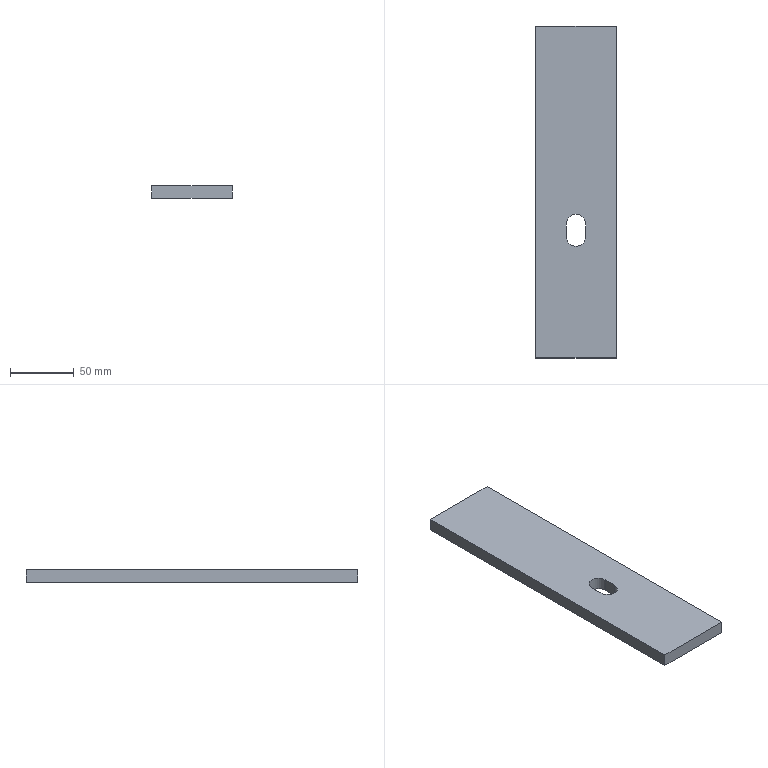Part | STEP file | E3-计量楼梯连接Plate 1 | 1 solid | 10 faces | box 63 x 260 x 10 mm | volume 160533 mm3 | plane 8 | cylinder 2 | commonest cylinder face diameters 15 x2
STEP:
#1=CARTESIAN_POINT('',(0.,0.,0.));
#2=DIRECTION('',(0.,0.,1.));
#3=DIRECTION('',(1.,0.,0.));
#4=AXIS2_PLACEMENT_3D('',#1,#2,#3);
#5=CARTESIAN_POINT('',(-31.5,260.,0.));
#6=VERTEX_POINT('',#5);
#7=CARTESIAN_POINT('',(-31.5,0.,0.));
#8=VERTEX_POINT('',#7);
#9=CARTESIAN_POINT('',(-31.5,260.,0.));
#10=DIRECTION('',(0.,-1.,0.));
#11=VECTOR('',#10,1.);
#12=LINE('',#9,#11);
#13=CARTESIAN_POINT('',(-31.5,260.,-10.));
#14=DIRECTION('',(1.,0.,0.));
#15=DIRECTION('',(0.,1.,0.));
#16=AXIS2_PLACEMENT_3D('',#13,#14,#15);
#17=PLANE('',#16);
#18=CARTESIAN_POINT('',(0.,10.));
#19=DIRECTION('',(-1.,0.));
#20=VECTOR('',#19,1.);
#21=LINE('',#18,#20);
#22=(GEOMETRIC_REPRESENTATION_CONTEXT(2)PARAMETRIC_REPRESENTATION_CONTEXT()REPRESENTATION_CONTEXT('',''));
#23=DEFINITIONAL_REPRESENTATION('',(#21),#22);
#24=PCURVE('',#17,#23);
#25=CARTESIAN_POINT('',(0.,0.,0.));
#26=DIRECTION('',(0.,0.,-1.));
#27=DIRECTION('',(1.,0.,0.));
#28=AXIS2_PLACEMENT_3D('',#25,#26,#27);
#29=PLANE('',#28);
#30=CARTESIAN_POINT('',(-31.5,-260.));
#31=DIRECTION('',(0.,1.));
#32=VECTOR('',#31,1.);
#33=LINE('',#30,#32);
#34=(GEOMETRIC_REPRESENTATION_CONTEXT(2)PARAMETRIC_REPRESENTATION_CONTEXT()REPRESENTATION_CONTEXT('',''));
#35=DEFINITIONAL_REPRESENTATION('',(#33),#34);
#36=PCURVE('',#29,#35);
#37=SURFACE_CURVE('',#12,(#24,#36),.PCURVE_S1.);
#38=EDGE_CURVE('',#6,#8,#37,.T.);
#39=ORIENTED_EDGE('',*,*,#38,.F.);
#40=CARTESIAN_POINT('',(-31.5,260.,-10.));
#41=VERTEX_POINT('',#40);
#42=CARTESIAN_POINT('',(-31.5,260.,-10.));
#43=DIRECTION('',(0.,0.,1.));
#44=VECTOR('',#43,1.);
#45=LINE('',#42,#44);
#46=CARTESIAN_POINT('',(0.,0.));
#47=DIRECTION('',(0.,1.));
#48=VECTOR('',#47,1.);
#49=LINE('',#46,#48);
#50=(GEOMETRIC_REPRESENTATION_CONTEXT(2)PARAMETRIC_REPRESENTATION_CONTEXT()REPRESENTATION_CONTEXT('',''));
#51=DEFINITIONAL_REPRESENTATION('',(#49),#50);
#52=PCURVE('',#17,#51);
#53=CARTESIAN_POINT('',(-31.5,260.,-10.));
#54=DIRECTION('',(0.,-1.,0.));
#55=DIRECTION('',(0.,0.,1.));
#56=AXIS2_PLACEMENT_3D('',#53,#54,#55);
#57=PLANE('',#56);
#58=CARTESIAN_POINT('',(0.,0.));
#59=DIRECTION('',(1.,0.));
#60=VECTOR('',#59,1.);
#61=LINE('',#58,#60);
#62=(GEOMETRIC_REPRESENTATION_CONTEXT(2)PARAMETRIC_REPRESENTATION_CONTEXT()REPRESENTATION_CONTEXT('',''));
#63=DEFINITIONAL_REPRESENTATION('',(#61),#62);
#64=PCURVE('',#57,#63);
#65=SURFACE_CURVE('',#45,(#52,#64),.PCURVE_S1.);
#66=EDGE_CURVE('',#41,#6,#65,.T.);
#67=ORIENTED_EDGE('',*,*,#66,.F.);
#68=CARTESIAN_POINT('',(-31.5,0.,-10.));
#69=VERTEX_POINT('',#68);
#70=CARTESIAN_POINT('',(-31.5,260.,-10.));
#71=DIRECTION('',(0.,-1.,0.));
#72=VECTOR('',#71,1.);
#73=LINE('',#70,#72);
#74=CARTESIAN_POINT('',(0.,0.));
#75=DIRECTION('',(-1.,0.));
#76=VECTOR('',#75,1.);
#77=LINE('',#74,#76);
#78=(GEOMETRIC_REPRESENTATION_CONTEXT(2)PARAMETRIC_REPRESENTATION_CONTEXT()REPRESENTATION_CONTEXT('',''));
#79=DEFINITIONAL_REPRESENTATION('',(#77),#78);
#80=PCURVE('',#17,#79);
#81=CARTESIAN_POINT('',(0.,0.,-10.));
#82=DIRECTION('',(0.,0.,-1.));
#83=DIRECTION('',(1.,0.,0.));
#84=AXIS2_PLACEMENT_3D('',#81,#82,#83);
#85=PLANE('',#84);
#86=CARTESIAN_POINT('',(-31.5,-260.));
#87=DIRECTION('',(0.,1.));
#88=VECTOR('',#87,1.);
#89=LINE('',#86,#88);
#90=(GEOMETRIC_REPRESENTATION_CONTEXT(2)PARAMETRIC_REPRESENTATION_CONTEXT()REPRESENTATION_CONTEXT('',''));
#91=DEFINITIONAL_REPRESENTATION('',(#89),#90);
#92=PCURVE('',#85,#91);
#93=SURFACE_CURVE('',#73,(#80,#92),.PCURVE_S1.);
#94=EDGE_CURVE('',#41,#69,#93,.T.);
#95=ORIENTED_EDGE('',*,*,#94,.T.);
#96=CARTESIAN_POINT('',(-31.5,0.,-10.));
#97=DIRECTION('',(0.,0.,1.));
#98=VECTOR('',#97,1.);
#99=LINE('',#96,#98);
#100=CARTESIAN_POINT('',(-260.,0.));
#101=DIRECTION('',(0.,1.));
#102=VECTOR('',#101,1.);
#103=LINE('',#100,#102);
#104=(GEOMETRIC_REPRESENTATION_CONTEXT(2)PARAMETRIC_REPRESENTATION_CONTEXT()REPRESENTATION_CONTEXT('',''));
#105=DEFINITIONAL_REPRESENTATION('',(#103),#104);
#106=PCURVE('',#17,#105);
#107=CARTESIAN_POINT('',(-31.5,0.,-10.));
#108=DIRECTION('',(0.,1.,0.));
#109=DIRECTION('',(0.,0.,-1.));
#110=AXIS2_PLACEMENT_3D('',#107,#108,#109);
#111=PLANE('',#110);
#112=CARTESIAN_POINT('',(0.,0.));
#113=DIRECTION('',(-1.,0.));
#114=VECTOR('',#113,1.);
#115=LINE('',#112,#114);
#116=(GEOMETRIC_REPRESENTATION_CONTEXT(2)PARAMETRIC_REPRESENTATION_CONTEXT()REPRESENTATION_CONTEXT('',''));
#117=DEFINITIONAL_REPRESENTATION('',(#115),#116);
#118=PCURVE('',#111,#117);
#119=SURFACE_CURVE('',#99,(#106,#118),.PCURVE_S1.);
#120=EDGE_CURVE('',#69,#8,#119,.T.);
#121=ORIENTED_EDGE('',*,*,#120,.T.);
#122=EDGE_LOOP('',(#39,#67,#95,#121));
#123=FACE_BOUND('',#122,.T.);
#124=ADVANCED_FACE('',(#123),#17,.F.);
#125=CARTESIAN_POINT('',(31.5,0.,0.));
#126=VERTEX_POINT('',#125);
#127=CARTESIAN_POINT('',(-31.5,0.,0.));
#128=DIRECTION('',(1.,0.,0.));
#129=VECTOR('',#128,1.);
#130=LINE('',#127,#129);
#131=CARTESIAN_POINT('',(-10.,0.));
#132=DIRECTION('',(0.,-1.));
#133=VECTOR('',#132,1.);
#134=LINE('',#131,#133);
#135=(GEOMETRIC_REPRESENTATION_CONTEXT(2)PARAMETRIC_REPRESENTATION_CONTEXT()REPRESENTATION_CONTEXT('',''));
#136=DEFINITIONAL_REPRESENTATION('',(#134),#135);
#137=PCURVE('',#111,#136);
#138=CARTESIAN_POINT('',(-31.5,0.));
#139=DIRECTION('',(1.,0.));
#140=VECTOR('',#139,1.);
#141=LINE('',#138,#140);
#142=(GEOMETRIC_REPRESENTATION_CONTEXT(2)PARAMETRIC_REPRESENTATION_CONTEXT()REPRESENTATION_CONTEXT('',''));
#143=DEFINITIONAL_REPRESENTATION('',(#141),#142);
#144=PCURVE('',#29,#143);
#145=SURFACE_CURVE('',#130,(#137,#144),.PCURVE_S1.);
#146=EDGE_CURVE('',#8,#126,#145,.T.);
#147=ORIENTED_EDGE('',*,*,#146,.F.);
#148=ORIENTED_EDGE('',*,*,#120,.F.);
#149=CARTESIAN_POINT('',(31.5,0.,-10.));
#150=VERTEX_POINT('',#149);
#151=CARTESIAN_POINT('',(-31.5,0.,-10.));
#152=DIRECTION('',(1.,0.,0.));
#153=VECTOR('',#152,1.);
#154=LINE('',#151,#153);
#155=CARTESIAN_POINT('',(0.,0.));
#156=DIRECTION('',(0.,-1.));
#157=VECTOR('',#156,1.);
#158=LINE('',#155,#157);
#159=(GEOMETRIC_REPRESENTATION_CONTEXT(2)PARAMETRIC_REPRESENTATION_CONTEXT()REPRESENTATION_CONTEXT('',''));
#160=DEFINITIONAL_REPRESENTATION('',(#158),#159);
#161=PCURVE('',#111,#160);
#162=CARTESIAN_POINT('',(-31.5,0.));
#163=DIRECTION('',(1.,0.));
#164=VECTOR('',#163,1.);
#165=LINE('',#162,#164);
#166=(GEOMETRIC_REPRESENTATION_CONTEXT(2)PARAMETRIC_REPRESENTATION_CONTEXT()REPRESENTATION_CONTEXT('',''));
#167=DEFINITIONAL_REPRESENTATION('',(#165),#166);
#168=PCURVE('',#85,#167);
#169=SURFACE_CURVE('',#154,(#161,#168),.PCURVE_S1.);
#170=EDGE_CURVE('',#69,#150,#169,.T.);
#171=ORIENTED_EDGE('',*,*,#170,.T.);
#172=CARTESIAN_POINT('',(31.5,0.,-10.));
#173=DIRECTION('',(0.,0.,1.));
#174=VECTOR('',#173,1.);
#175=LINE('',#172,#174);
#176=CARTESIAN_POINT('',(0.,-63.));
#177=DIRECTION('',(-1.,0.));
#178=VECTOR('',#177,1.);
#179=LINE('',#176,#178);
#180=(GEOMETRIC_REPRESENTATION_CONTEXT(2)PARAMETRIC_REPRESENTATION_CONTEXT()REPRESENTATION_CONTEXT('',''));
#181=DEFINITIONAL_REPRESENTATION('',(#179),#180);
#182=PCURVE('',#111,#181);
#183=CARTESIAN_POINT('',(31.5,260.,-10.));
#184=DIRECTION('',(-1.,0.,0.));
#185=DIRECTION('',(0.,-1.,0.));
#186=AXIS2_PLACEMENT_3D('',#183,#184,#185);
#187=PLANE('',#186);
#188=CARTESIAN_POINT('',(260.,0.));
#189=DIRECTION('',(0.,1.));
#190=VECTOR('',#189,1.);
#191=LINE('',#188,#190);
#192=(GEOMETRIC_REPRESENTATION_CONTEXT(2)PARAMETRIC_REPRESENTATION_CONTEXT()REPRESENTATION_CONTEXT('',''));
#193=DEFINITIONAL_REPRESENTATION('',(#191),#192);
#194=PCURVE('',#187,#193);
#195=SURFACE_CURVE('',#175,(#182,#194),.PCURVE_S1.);
#196=EDGE_CURVE('',#150,#126,#195,.T.);
#197=ORIENTED_EDGE('',*,*,#196,.T.);
#198=EDGE_LOOP('',(#147,#148,#171,#197));
#199=FACE_BOUND('',#198,.T.);
#200=ADVANCED_FACE('',(#199),#111,.F.);
#201=CARTESIAN_POINT('',(31.5,260.,0.));
#202=VERTEX_POINT('',#201);
#203=CARTESIAN_POINT('',(31.5,260.,0.));
#204=DIRECTION('',(0.,1.,0.));
#205=VECTOR('',#204,1.);
#206=LINE('',#203,#205);
#207=CARTESIAN_POINT('',(0.,10.));
#208=DIRECTION('',(-1.,0.));
#209=VECTOR('',#208,1.);
#210=LINE('',#207,#209);
#211=(GEOMETRIC_REPRESENTATION_CONTEXT(2)PARAMETRIC_REPRESENTATION_CONTEXT()REPRESENTATION_CONTEXT('',''));
#212=DEFINITIONAL_REPRESENTATION('',(#210),#211);
#213=PCURVE('',#187,#212);
#214=CARTESIAN_POINT('',(31.5,-260.));
#215=DIRECTION('',(0.,-1.));
#216=VECTOR('',#215,1.);
#217=LINE('',#214,#216);
#218=(GEOMETRIC_REPRESENTATION_CONTEXT(2)PARAMETRIC_REPRESENTATION_CONTEXT()REPRESENTATION_CONTEXT('',''));
#219=DEFINITIONAL_REPRESENTATION('',(#217),#218);
#220=PCURVE('',#29,#219);
#221=SURFACE_CURVE('',#206,(#213,#220),.PCURVE_S1.);
#222=EDGE_CURVE('',#126,#202,#221,.T.);
#223=ORIENTED_EDGE('',*,*,#222,.F.);
#224=ORIENTED_EDGE('',*,*,#196,.F.);
#225=CARTESIAN_POINT('',(31.5,260.,-10.));
#226=VERTEX_POINT('',#225);
#227=CARTESIAN_POINT('',(31.5,260.,-10.));
#228=DIRECTION('',(0.,1.,0.));
#229=VECTOR('',#228,1.);
#230=LINE('',#227,#229);
#231=CARTESIAN_POINT('',(0.,0.));
#232=DIRECTION('',(-1.,0.));
#233=VECTOR('',#232,1.);
#234=LINE('',#231,#233);
#235=(GEOMETRIC_REPRESENTATION_CONTEXT(2)PARAMETRIC_REPRESENTATION_CONTEXT()REPRESENTATION_CONTEXT('',''));
#236=DEFINITIONAL_REPRESENTATION('',(#234),#235);
#237=PCURVE('',#187,#236);
#238=CARTESIAN_POINT('',(31.5,-260.));
#239=DIRECTION('',(0.,-1.));
#240=VECTOR('',#239,1.);
#241=LINE('',#238,#240);
#242=(GEOMETRIC_REPRESENTATION_CONTEXT(2)PARAMETRIC_REPRESENTATION_CONTEXT()REPRESENTATION_CONTEXT('',''));
#243=DEFINITIONAL_REPRESENTATION('',(#241),#242);
#244=PCURVE('',#85,#243);
#245=SURFACE_CURVE('',#230,(#237,#244),.PCURVE_S1.);
#246=EDGE_CURVE('',#150,#226,#245,.T.);
#247=ORIENTED_EDGE('',*,*,#246,.T.);
#248=CARTESIAN_POINT('',(31.5,260.,-10.));
#249=DIRECTION('',(0.,0.,1.));
#250=VECTOR('',#249,1.);
#251=LINE('',#248,#250);
#252=CARTESIAN_POINT('',(0.,0.));
#253=DIRECTION('',(0.,1.));
#254=VECTOR('',#253,1.);
#255=LINE('',#252,#254);
#256=(GEOMETRIC_REPRESENTATION_CONTEXT(2)PARAMETRIC_REPRESENTATION_CONTEXT()REPRESENTATION_CONTEXT('',''));
#257=DEFINITIONAL_REPRESENTATION('',(#255),#256);
#258=PCURVE('',#187,#257);
#259=CARTESIAN_POINT('',(0.,-63.));
#260=DIRECTION('',(1.,0.));
#261=VECTOR('',#260,1.);
#262=LINE('',#259,#261);
#263=(GEOMETRIC_REPRESENTATION_CONTEXT(2)PARAMETRIC_REPRESENTATION_CONTEXT()REPRESENTATION_CONTEXT('',''));
#264=DEFINITIONAL_REPRESENTATION('',(#262),#263);
#265=PCURVE('',#57,#264);
#266=SURFACE_CURVE('',#251,(#258,#265),.PCURVE_S1.);
#267=EDGE_CURVE('',#226,#202,#266,.T.);
#268=ORIENTED_EDGE('',*,*,#267,.T.);
#269=EDGE_LOOP('',(#223,#224,#247,#268));
#270=FACE_BOUND('',#269,.T.);
#271=ADVANCED_FACE('',(#270),#187,.F.);
#272=CARTESIAN_POINT('',(-31.5,260.,0.));
#273=DIRECTION('',(-1.,0.,0.));
#274=VECTOR('',#273,1.);
#275=LINE('',#272,#274);
#276=CARTESIAN_POINT('',(10.,0.));
#277=DIRECTION('',(0.,1.));
#278=VECTOR('',#277,1.);
#279=LINE('',#276,#278);
#280=(GEOMETRIC_REPRESENTATION_CONTEXT(2)PARAMETRIC_REPRESENTATION_CONTEXT()REPRESENTATION_CONTEXT('',''));
#281=DEFINITIONAL_REPRESENTATION('',(#279),#280);
#282=PCURVE('',#57,#281);
#283=CARTESIAN_POINT('',(-31.5,-260.));
#284=DIRECTION('',(-1.,0.));
#285=VECTOR('',#284,1.);
#286=LINE('',#283,#285);
#287=(GEOMETRIC_REPRESENTATION_CONTEXT(2)PARAMETRIC_REPRESENTATION_CONTEXT()REPRESENTATION_CONTEXT('',''));
#288=DEFINITIONAL_REPRESENTATION('',(#286),#287);
#289=PCURVE('',#29,#288);
#290=SURFACE_CURVE('',#275,(#282,#289),.PCURVE_S1.);
#291=EDGE_CURVE('',#202,#6,#290,.T.);
#292=ORIENTED_EDGE('',*,*,#291,.F.);
#293=ORIENTED_EDGE('',*,*,#267,.F.);
#294=CARTESIAN_POINT('',(-31.5,260.,-10.));
#295=DIRECTION('',(-1.,0.,0.));
#296=VECTOR('',#295,1.);
#297=LINE('',#294,#296);
#298=CARTESIAN_POINT('',(0.,0.));
#299=DIRECTION('',(0.,1.));
#300=VECTOR('',#299,1.);
#301=LINE('',#298,#300);
#302=(GEOMETRIC_REPRESENTATION_CONTEXT(2)PARAMETRIC_REPRESENTATION_CONTEXT()REPRESENTATION_CONTEXT('',''));
#303=DEFINITIONAL_REPRESENTATION('',(#301),#302);
#304=PCURVE('',#57,#303);
#305=CARTESIAN_POINT('',(-31.5,-260.));
#306=DIRECTION('',(-1.,0.));
#307=VECTOR('',#306,1.);
#308=LINE('',#305,#307);
#309=(GEOMETRIC_REPRESENTATION_CONTEXT(2)PARAMETRIC_REPRESENTATION_CONTEXT()REPRESENTATION_CONTEXT('',''));
#310=DEFINITIONAL_REPRESENTATION('',(#308),#309);
#311=PCURVE('',#85,#310);
#312=SURFACE_CURVE('',#297,(#304,#311),.PCURVE_S1.);
#313=EDGE_CURVE('',#226,#41,#312,.T.);
#314=ORIENTED_EDGE('',*,*,#313,.T.);
#315=ORIENTED_EDGE('',*,*,#66,.T.);
#316=EDGE_LOOP('',(#292,#293,#314,#315));
#317=FACE_BOUND('',#316,.T.);
#318=ADVANCED_FACE('',(#317),#57,.F.);
#319=CARTESIAN_POINT('',(7.5,95.,-10.));
#320=VERTEX_POINT('',#319);
#321=CARTESIAN_POINT('',(7.5,105.,-10.));
#322=VERTEX_POINT('',#321);
#323=CARTESIAN_POINT('',(7.5,95.,-10.));
#324=DIRECTION('',(0.,1.,0.));
#325=VECTOR('',#324,1.);
#326=LINE('',#323,#325);
#327=CARTESIAN_POINT('',(7.5,-95.));
#328=DIRECTION('',(0.,-1.));
#329=VECTOR('',#328,1.);
#330=LINE('',#327,#329);
#331=(GEOMETRIC_REPRESENTATION_CONTEXT(2)PARAMETRIC_REPRESENTATION_CONTEXT()REPRESENTATION_CONTEXT('',''));
#332=DEFINITIONAL_REPRESENTATION('',(#330),#331);
#333=PCURVE('',#85,#332);
#334=CARTESIAN_POINT('',(7.5,95.,0.001));
#335=DIRECTION('',(1.,0.,0.));
#336=DIRECTION('',(0.,1.,0.));
#337=AXIS2_PLACEMENT_3D('',#334,#335,#336);
#338=PLANE('',#337);
#339=CARTESIAN_POINT('',(0.,-10.001));
#340=DIRECTION('',(1.,0.));
#341=VECTOR('',#340,1.);
#342=LINE('',#339,#341);
#343=(GEOMETRIC_REPRESENTATION_CONTEXT(2)PARAMETRIC_REPRESENTATION_CONTEXT()REPRESENTATION_CONTEXT('',''));
#344=DEFINITIONAL_REPRESENTATION('',(#342),#343);
#345=PCURVE('',#338,#344);
#346=SURFACE_CURVE('',#326,(#333,#345),.PCURVE_S1.);
#347=EDGE_CURVE('',#320,#322,#346,.T.);
#348=ORIENTED_EDGE('',*,*,#347,.T.);
#349=CARTESIAN_POINT('',(-7.5,105.,-10.));
#350=VERTEX_POINT('',#349);
#351=CARTESIAN_POINT('',(0.,105.,-10.));
#352=DIRECTION('',(0.,0.,1.));
#353=DIRECTION('',(1.,0.,0.));
#354=AXIS2_PLACEMENT_3D('',#351,#352,#353);
#355=CIRCLE('',#354,7.5);
#356=CARTESIAN_POINT('',(7.5,-105.));
#357=CARTESIAN_POINT('',(7.5,-117.99));
#358=CARTESIAN_POINT('',(-3.75,-111.495));
#359=CARTESIAN_POINT('',(-15.,-105.));
#360=CARTESIAN_POINT('',(-3.75,-98.505));
#361=CARTESIAN_POINT('',(7.5,-92.01));
#362=CARTESIAN_POINT('',(7.5,-105.));
#363=(BOUNDED_CURVE()B_SPLINE_CURVE(2,(#356,#357,#358,#359,#360,#361,#362),.UNSPECIFIED.,.T.,.F.)B_SPLINE_CURVE_WITH_KNOTS((1,2,2,2,2,1),(-2.094,0.,2.094,4.189,6.283,8.378),.UNSPECIFIED.)CURVE()GEOMETRIC_REPRESENTATION_ITEM()RATIONAL_B_SPLINE_CURVE((1.,0.5,1.,0.5,1.,0.5,1.))REPRESENTATION_ITEM(''));
#364=(GEOMETRIC_REPRESENTATION_CONTEXT(2)PARAMETRIC_REPRESENTATION_CONTEXT()REPRESENTATION_CONTEXT('',''));
#365=DEFINITIONAL_REPRESENTATION('',(#363),#364);
#366=PCURVE('',#85,#365);
#367=CARTESIAN_POINT('',(0.,105.,-10.));
#368=DIRECTION('',(0.,0.,-1.));
#369=DIRECTION('',(1.,0.,0.));
#370=AXIS2_PLACEMENT_3D('',#367,#368,#369);
#371=CYLINDRICAL_SURFACE('',#370,7.5);
#372=CARTESIAN_POINT('',(6.283,0.));
#373=DIRECTION('',(-1.,0.));
#374=VECTOR('',#373,1.);
#375=LINE('',#372,#374);
#376=(GEOMETRIC_REPRESENTATION_CONTEXT(2)PARAMETRIC_REPRESENTATION_CONTEXT()REPRESENTATION_CONTEXT('',''));
#377=DEFINITIONAL_REPRESENTATION('',(#375),#376);
#378=PCURVE('',#371,#377);
#379=SURFACE_CURVE('',#355,(#366,#378),.PCURVE_S1.);
#380=EDGE_CURVE('',#322,#350,#379,.T.);
#381=ORIENTED_EDGE('',*,*,#380,.T.);
#382=CARTESIAN_POINT('',(-7.5,95.,-10.));
#383=VERTEX_POINT('',#382);
#384=CARTESIAN_POINT('',(-7.5,95.,-10.));
#385=DIRECTION('',(0.,1.,0.));
#386=VECTOR('',#385,1.);
#387=LINE('',#384,#386);
#388=CARTESIAN_POINT('',(-7.5,-95.));
#389=DIRECTION('',(0.,-1.));
#390=VECTOR('',#389,1.);
#391=LINE('',#388,#390);
#392=(GEOMETRIC_REPRESENTATION_CONTEXT(2)PARAMETRIC_REPRESENTATION_CONTEXT()REPRESENTATION_CONTEXT('',''));
#393=DEFINITIONAL_REPRESENTATION('',(#391),#392);
#394=PCURVE('',#85,#393);
#395=CARTESIAN_POINT('',(-7.5,95.,-10.));
#396=DIRECTION('',(-1.,0.,0.));
#397=DIRECTION('',(0.,-1.,0.));
#398=AXIS2_PLACEMENT_3D('',#395,#396,#397);
#399=PLANE('',#398);
#400=CARTESIAN_POINT('',(0.,0.));
#401=DIRECTION('',(-1.,0.));
#402=VECTOR('',#401,1.);
#403=LINE('',#400,#402);
#404=(GEOMETRIC_REPRESENTATION_CONTEXT(2)PARAMETRIC_REPRESENTATION_CONTEXT()REPRESENTATION_CONTEXT('',''));
#405=DEFINITIONAL_REPRESENTATION('',(#403),#404);
#406=PCURVE('',#399,#405);
#407=SURFACE_CURVE('',#387,(#394,#406),.PCURVE_S1.);
#408=EDGE_CURVE('',#383,#350,#407,.T.);
#409=ORIENTED_EDGE('',*,*,#408,.F.);
#410=CARTESIAN_POINT('',(0.,95.,-10.));
#411=DIRECTION('',(0.,0.,1.));
#412=DIRECTION('',(1.,0.,0.));
#413=AXIS2_PLACEMENT_3D('',#410,#411,#412);
#414=CIRCLE('',#413,7.5);
#415=CARTESIAN_POINT('',(7.5,-95.));
#416=CARTESIAN_POINT('',(7.5,-107.99));
#417=CARTESIAN_POINT('',(-3.75,-101.495));
#418=CARTESIAN_POINT('',(-15.,-95.));
#419=CARTESIAN_POINT('',(-3.75,-88.505));
#420=CARTESIAN_POINT('',(7.5,-82.01));
#421=CARTESIAN_POINT('',(7.5,-95.));
#422=(BOUNDED_CURVE()B_SPLINE_CURVE(2,(#415,#416,#417,#418,#419,#420,#421),.UNSPECIFIED.,.T.,.F.)B_SPLINE_CURVE_WITH_KNOTS((1,2,2,2,2,1),(-2.094,0.,2.094,4.189,6.283,8.378),.UNSPECIFIED.)CURVE()GEOMETRIC_REPRESENTATION_ITEM()RATIONAL_B_SPLINE_CURVE((1.,0.5,1.,0.5,1.,0.5,1.))REPRESENTATION_ITEM(''));
#423=(GEOMETRIC_REPRESENTATION_CONTEXT(2)PARAMETRIC_REPRESENTATION_CONTEXT()REPRESENTATION_CONTEXT('',''));
#424=DEFINITIONAL_REPRESENTATION('',(#422),#423);
#425=PCURVE('',#85,#424);
#426=CARTESIAN_POINT('',(0.,95.,-10.));
#427=DIRECTION('',(0.,0.,-1.));
#428=DIRECTION('',(1.,0.,0.));
#429=AXIS2_PLACEMENT_3D('',#426,#427,#428);
#430=CYLINDRICAL_SURFACE('',#429,7.5);
#431=CARTESIAN_POINT('',(6.283,0.));
#432=DIRECTION('',(-1.,0.));
#433=VECTOR('',#432,1.);
#434=LINE('',#431,#433);
#435=(GEOMETRIC_REPRESENTATION_CONTEXT(2)PARAMETRIC_REPRESENTATION_CONTEXT()REPRESENTATION_CONTEXT('',''));
#436=DEFINITIONAL_REPRESENTATION('',(#434),#435);
#437=PCURVE('',#430,#436);
#438=SURFACE_CURVE('',#414,(#425,#437),.PCURVE_S1.);
#439=EDGE_CURVE('',#383,#320,#438,.T.);
#440=ORIENTED_EDGE('',*,*,#439,.T.);
#441=EDGE_LOOP('',(#348,#381,#409,#440));
#442=FACE_BOUND('',#441,.T.);
#443=ORIENTED_EDGE('',*,*,#94,.F.);
#444=ORIENTED_EDGE('',*,*,#313,.F.);
#445=ORIENTED_EDGE('',*,*,#246,.F.);
#446=ORIENTED_EDGE('',*,*,#170,.F.);
#447=EDGE_LOOP('',(#443,#444,#445,#446));
#448=FACE_BOUND('',#447,.T.);
#449=ADVANCED_FACE('',(#442,#448),#85,.T.);
#450=CARTESIAN_POINT('',(7.5,105.,0.));
#451=VERTEX_POINT('',#450);
#452=CARTESIAN_POINT('',(-7.5,105.,0.));
#453=VERTEX_POINT('',#452);
#454=CARTESIAN_POINT('',(0.,105.,0.));
#455=DIRECTION('',(0.,0.,1.));
#456=DIRECTION('',(1.,0.,0.));
#457=AXIS2_PLACEMENT_3D('',#454,#455,#456);
#458=CIRCLE('',#457,7.5);
#459=CARTESIAN_POINT('',(7.5,-105.));
#460=CARTESIAN_POINT('',(7.5,-117.99));
#461=CARTESIAN_POINT('',(-3.75,-111.495));
#462=CARTESIAN_POINT('',(-15.,-105.));
#463=CARTESIAN_POINT('',(-3.75,-98.505));
#464=CARTESIAN_POINT('',(7.5,-92.01));
#465=CARTESIAN_POINT('',(7.5,-105.));
#466=(BOUNDED_CURVE()B_SPLINE_CURVE(2,(#459,#460,#461,#462,#463,#464,#465),.UNSPECIFIED.,.T.,.F.)B_SPLINE_CURVE_WITH_KNOTS((1,2,2,2,2,1),(-2.094,0.,2.094,4.189,6.283,8.378),.UNSPECIFIED.)CURVE()GEOMETRIC_REPRESENTATION_ITEM()RATIONAL_B_SPLINE_CURVE((1.,0.5,1.,0.5,1.,0.5,1.))REPRESENTATION_ITEM(''));
#467=(GEOMETRIC_REPRESENTATION_CONTEXT(2)PARAMETRIC_REPRESENTATION_CONTEXT()REPRESENTATION_CONTEXT('',''));
#468=DEFINITIONAL_REPRESENTATION('',(#466),#467);
#469=PCURVE('',#29,#468);
#470=CARTESIAN_POINT('',(6.283,-10.));
#471=DIRECTION('',(-1.,0.));
#472=VECTOR('',#471,1.);
#473=LINE('',#470,#472);
#474=(GEOMETRIC_REPRESENTATION_CONTEXT(2)PARAMETRIC_REPRESENTATION_CONTEXT()REPRESENTATION_CONTEXT('',''));
#475=DEFINITIONAL_REPRESENTATION('',(#473),#474);
#476=PCURVE('',#371,#475);
#477=SURFACE_CURVE('',#458,(#469,#476),.PCURVE_S1.);
#478=EDGE_CURVE('',#451,#453,#477,.T.);
#479=ORIENTED_EDGE('',*,*,#478,.F.);
#480=CARTESIAN_POINT('',(7.5,95.,0.));
#481=VERTEX_POINT('',#480);
#482=CARTESIAN_POINT('',(7.5,0.,0.));
#483=DIRECTION('',(0.,1.,0.));
#484=VECTOR('',#483,1.);
#485=LINE('',#482,#484);
#486=CARTESIAN_POINT('',(7.5,0.));
#487=DIRECTION('',(0.,-1.));
#488=VECTOR('',#487,1.);
#489=LINE('',#486,#488);
#490=(GEOMETRIC_REPRESENTATION_CONTEXT(2)PARAMETRIC_REPRESENTATION_CONTEXT()REPRESENTATION_CONTEXT('',''));
#491=DEFINITIONAL_REPRESENTATION('',(#489),#490);
#492=PCURVE('',#29,#491);
#493=CARTESIAN_POINT('',(-95.,-0.001));
#494=DIRECTION('',(1.,0.));
#495=VECTOR('',#494,1.);
#496=LINE('',#493,#495);
#497=(GEOMETRIC_REPRESENTATION_CONTEXT(2)PARAMETRIC_REPRESENTATION_CONTEXT()REPRESENTATION_CONTEXT('',''));
#498=DEFINITIONAL_REPRESENTATION('',(#496),#497);
#499=PCURVE('',#338,#498);
#500=SURFACE_CURVE('',#485,(#492,#499),.PCURVE_S1.);
#501=EDGE_CURVE('',#481,#451,#500,.T.);
#502=ORIENTED_EDGE('',*,*,#501,.F.);
#503=CARTESIAN_POINT('',(-7.5,95.,0.));
#504=VERTEX_POINT('',#503);
#505=CARTESIAN_POINT('',(0.,95.,0.));
#506=DIRECTION('',(0.,0.,1.));
#507=DIRECTION('',(1.,0.,0.));
#508=AXIS2_PLACEMENT_3D('',#505,#506,#507);
#509=CIRCLE('',#508,7.5);
#510=CARTESIAN_POINT('',(7.5,-95.));
#511=CARTESIAN_POINT('',(7.5,-107.99));
#512=CARTESIAN_POINT('',(-3.75,-101.495));
#513=CARTESIAN_POINT('',(-15.,-95.));
#514=CARTESIAN_POINT('',(-3.75,-88.505));
#515=CARTESIAN_POINT('',(7.5,-82.01));
#516=CARTESIAN_POINT('',(7.5,-95.));
#517=(BOUNDED_CURVE()B_SPLINE_CURVE(2,(#510,#511,#512,#513,#514,#515,#516),.UNSPECIFIED.,.T.,.F.)B_SPLINE_CURVE_WITH_KNOTS((1,2,2,2,2,1),(-2.094,0.,2.094,4.189,6.283,8.378),.UNSPECIFIED.)CURVE()GEOMETRIC_REPRESENTATION_ITEM()RATIONAL_B_SPLINE_CURVE((1.,0.5,1.,0.5,1.,0.5,1.))REPRESENTATION_ITEM(''));
#518=(GEOMETRIC_REPRESENTATION_CONTEXT(2)PARAMETRIC_REPRESENTATION_CONTEXT()REPRESENTATION_CONTEXT('',''));
#519=DEFINITIONAL_REPRESENTATION('',(#517),#518);
#520=PCURVE('',#29,#519);
#521=CARTESIAN_POINT('',(6.283,-10.));
#522=DIRECTION('',(-1.,0.));
#523=VECTOR('',#522,1.);
#524=LINE('',#521,#523);
#525=(GEOMETRIC_REPRESENTATION_CONTEXT(2)PARAMETRIC_REPRESENTATION_CONTEXT()REPRESENTATION_CONTEXT('',''));
#526=DEFINITIONAL_REPRESENTATION('',(#524),#525);
#527=PCURVE('',#430,#526);
#528=SURFACE_CURVE('',#509,(#520,#527),.PCURVE_S1.);
#529=EDGE_CURVE('',#504,#481,#528,.T.);
#530=ORIENTED_EDGE('',*,*,#529,.F.);
#531=CARTESIAN_POINT('',(-7.5,0.,0.));
#532=DIRECTION('',(0.,-1.,0.));
#533=VECTOR('',#532,1.);
#534=LINE('',#531,#533);
#535=CARTESIAN_POINT('',(-7.5,0.));
#536=DIRECTION('',(0.,1.));
#537=VECTOR('',#536,1.);
#538=LINE('',#535,#537);
#539=(GEOMETRIC_REPRESENTATION_CONTEXT(2)PARAMETRIC_REPRESENTATION_CONTEXT()REPRESENTATION_CONTEXT('',''));
#540=DEFINITIONAL_REPRESENTATION('',(#538),#539);
#541=PCURVE('',#29,#540);
#542=CARTESIAN_POINT('',(95.,10.));
#543=DIRECTION('',(1.,0.));
#544=VECTOR('',#543,1.);
#545=LINE('',#542,#544);
#546=(GEOMETRIC_REPRESENTATION_CONTEXT(2)PARAMETRIC_REPRESENTATION_CONTEXT()REPRESENTATION_CONTEXT('',''));
#547=DEFINITIONAL_REPRESENTATION('',(#545),#546);
#548=PCURVE('',#399,#547);
#549=SURFACE_CURVE('',#534,(#541,#548),.PCURVE_S1.);
#550=EDGE_CURVE('',#453,#504,#549,.T.);
#551=ORIENTED_EDGE('',*,*,#550,.F.);
#552=EDGE_LOOP('',(#479,#502,#530,#551));
#553=FACE_BOUND('',#552,.T.);
#554=ORIENTED_EDGE('',*,*,#38,.T.);
#555=ORIENTED_EDGE('',*,*,#146,.T.);
#556=ORIENTED_EDGE('',*,*,#222,.T.);
#557=ORIENTED_EDGE('',*,*,#291,.T.);
#558=EDGE_LOOP('',(#554,#555,#556,#557));
#559=FACE_BOUND('',#558,.T.);
#560=ADVANCED_FACE('',(#553,#559),#29,.F.);
#561=ORIENTED_EDGE('',*,*,#380,.T.);
#562=CARTESIAN_POINT('',(-7.5,105.,-10.));
#563=DIRECTION('',(0.,0.,-1.));
#564=VECTOR('',#563,1.);
#565=LINE('',#562,#564);
#566=CARTESIAN_POINT('',(3.142,0.));
#567=DIRECTION('',(0.,1.));
#568=VECTOR('',#567,1.);
#569=LINE('',#566,#568);
#570=(GEOMETRIC_REPRESENTATION_CONTEXT(2)PARAMETRIC_REPRESENTATION_CONTEXT()REPRESENTATION_CONTEXT('',''));
#571=DEFINITIONAL_REPRESENTATION('',(#569),#570);
#572=PCURVE('',#371,#571);
#573=CARTESIAN_POINT('',(-10.,0.));
#574=DIRECTION('',(0.,-1.));
#575=VECTOR('',#574,1.);
#576=LINE('',#573,#575);
#577=(GEOMETRIC_REPRESENTATION_CONTEXT(2)PARAMETRIC_REPRESENTATION_CONTEXT()REPRESENTATION_CONTEXT('',''));
#578=DEFINITIONAL_REPRESENTATION('',(#576),#577);
#579=PCURVE('',#399,#578);
#580=SURFACE_CURVE('',#565,(#572,#579),.PCURVE_S1.);
#581=EDGE_CURVE('',#453,#350,#580,.T.);
#582=ORIENTED_EDGE('',*,*,#581,.F.);
#583=ORIENTED_EDGE('',*,*,#478,.F.);
#584=CARTESIAN_POINT('',(7.5,105.,0.001));
#585=DIRECTION('',(0.,0.,1.));
#586=VECTOR('',#585,1.);
#587=LINE('',#584,#586);
#588=CARTESIAN_POINT('',(6.283,-10.001));
#589=DIRECTION('',(0.,-1.));
#590=VECTOR('',#589,1.);
#591=LINE('',#588,#590);
#592=(GEOMETRIC_REPRESENTATION_CONTEXT(2)PARAMETRIC_REPRESENTATION_CONTEXT()REPRESENTATION_CONTEXT('',''));
#593=DEFINITIONAL_REPRESENTATION('',(#591),#592);
#594=PCURVE('',#371,#593);
#595=CARTESIAN_POINT('',(10.,0.));
#596=DIRECTION('',(0.,1.));
#597=VECTOR('',#596,1.);
#598=LINE('',#595,#597);
#599=(GEOMETRIC_REPRESENTATION_CONTEXT(2)PARAMETRIC_REPRESENTATION_CONTEXT()REPRESENTATION_CONTEXT('',''));
#600=DEFINITIONAL_REPRESENTATION('',(#598),#599);
#601=PCURVE('',#338,#600);
#602=SURFACE_CURVE('',#587,(#594,#601),.PCURVE_S1.);
#603=EDGE_CURVE('',#322,#451,#602,.T.);
#604=ORIENTED_EDGE('',*,*,#603,.F.);
#605=EDGE_LOOP('',(#561,#582,#583,#604));
#606=FACE_BOUND('',#605,.F.);
#607=ADVANCED_FACE('',(#606),#371,.F.);
#608=ORIENTED_EDGE('',*,*,#439,.T.);
#609=CARTESIAN_POINT('',(7.5,95.,0.001));
#610=DIRECTION('',(0.,0.,1.));
#611=VECTOR('',#610,1.);
#612=LINE('',#609,#611);
#613=CARTESIAN_POINT('',(0.,-10.001));
#614=DIRECTION('',(0.,-1.));
#615=VECTOR('',#614,1.);
#616=LINE('',#613,#615);
#617=(GEOMETRIC_REPRESENTATION_CONTEXT(2)PARAMETRIC_REPRESENTATION_CONTEXT()REPRESENTATION_CONTEXT('',''));
#618=DEFINITIONAL_REPRESENTATION('',(#616),#617);
#619=PCURVE('',#430,#618);
#620=CARTESIAN_POINT('',(0.,0.));
#621=DIRECTION('',(0.,1.));
#622=VECTOR('',#621,1.);
#623=LINE('',#620,#622);
#624=(GEOMETRIC_REPRESENTATION_CONTEXT(2)PARAMETRIC_REPRESENTATION_CONTEXT()REPRESENTATION_CONTEXT('',''));
#625=DEFINITIONAL_REPRESENTATION('',(#623),#624);
#626=PCURVE('',#338,#625);
#627=SURFACE_CURVE('',#612,(#619,#626),.PCURVE_S1.);
#628=EDGE_CURVE('',#320,#481,#627,.T.);
#629=ORIENTED_EDGE('',*,*,#628,.T.);
#630=ORIENTED_EDGE('',*,*,#529,.F.);
#631=CARTESIAN_POINT('',(-7.5,95.,-10.));
#632=DIRECTION('',(0.,0.,1.));
#633=VECTOR('',#632,1.);
#634=LINE('',#631,#633);
#635=CARTESIAN_POINT('',(3.142,0.));
#636=DIRECTION('',(0.,-1.));
#637=VECTOR('',#636,1.);
#638=LINE('',#635,#637);
#639=(GEOMETRIC_REPRESENTATION_CONTEXT(2)PARAMETRIC_REPRESENTATION_CONTEXT()REPRESENTATION_CONTEXT('',''));
#640=DEFINITIONAL_REPRESENTATION('',(#638),#639);
#641=PCURVE('',#430,#640);
#642=CARTESIAN_POINT('',(0.,0.));
#643=DIRECTION('',(0.,1.));
#644=VECTOR('',#643,1.);
#645=LINE('',#642,#644);
#646=(GEOMETRIC_REPRESENTATION_CONTEXT(2)PARAMETRIC_REPRESENTATION_CONTEXT()REPRESENTATION_CONTEXT('',''));
#647=DEFINITIONAL_REPRESENTATION('',(#645),#646);
#648=PCURVE('',#399,#647);
#649=SURFACE_CURVE('',#634,(#641,#648),.PCURVE_S1.);
#650=EDGE_CURVE('',#383,#504,#649,.T.);
#651=ORIENTED_EDGE('',*,*,#650,.F.);
#652=EDGE_LOOP('',(#608,#629,#630,#651));
#653=FACE_BOUND('',#652,.F.);
#654=ADVANCED_FACE('',(#653),#430,.F.);
#655=ORIENTED_EDGE('',*,*,#581,.F.);
#656=ORIENTED_EDGE('',*,*,#550,.T.);
#657=ORIENTED_EDGE('',*,*,#650,.F.);
#658=ORIENTED_EDGE('',*,*,#408,.T.);
#659=EDGE_LOOP('',(#655,#656,#657,#658));
#660=FACE_BOUND('',#659,.T.);
#661=ADVANCED_FACE('',(#660),#399,.F.);
#662=ORIENTED_EDGE('',*,*,#628,.T.);
#663=ORIENTED_EDGE('',*,*,#501,.T.);
#664=ORIENTED_EDGE('',*,*,#603,.F.);
#665=ORIENTED_EDGE('',*,*,#347,.F.);
#666=EDGE_LOOP('',(#662,#663,#664,#665));
#667=FACE_BOUND('',#666,.T.);
#668=ADVANCED_FACE('',(#667),#338,.F.);
#669=CLOSED_SHELL('',(#124,#200,#271,#318,#449,#560,#607,#654,#661,#668));
#670=MANIFOLD_SOLID_BREP('',#669);
#671=(LENGTH_UNIT()NAMED_UNIT(*)SI_UNIT(.MILLI.,.METRE.));
#672=UNCERTAINTY_MEASURE_WITH_UNIT(LENGTH_MEASURE(0.0000001),#671,'','');
#673=(NAMED_UNIT(*)PLANE_ANGLE_UNIT()SI_UNIT($,.RADIAN.));
#674=(NAMED_UNIT(*)SI_UNIT($,.STERADIAN.)SOLID_ANGLE_UNIT());
#675=(GEOMETRIC_REPRESENTATION_CONTEXT(3)GLOBAL_UNCERTAINTY_ASSIGNED_CONTEXT((#672))GLOBAL_UNIT_ASSIGNED_CONTEXT((#671,#673,#674))REPRESENTATION_CONTEXT('',''));
#676=ADVANCED_BREP_SHAPE_REPRESENTATION('',(#4,#670),#675);